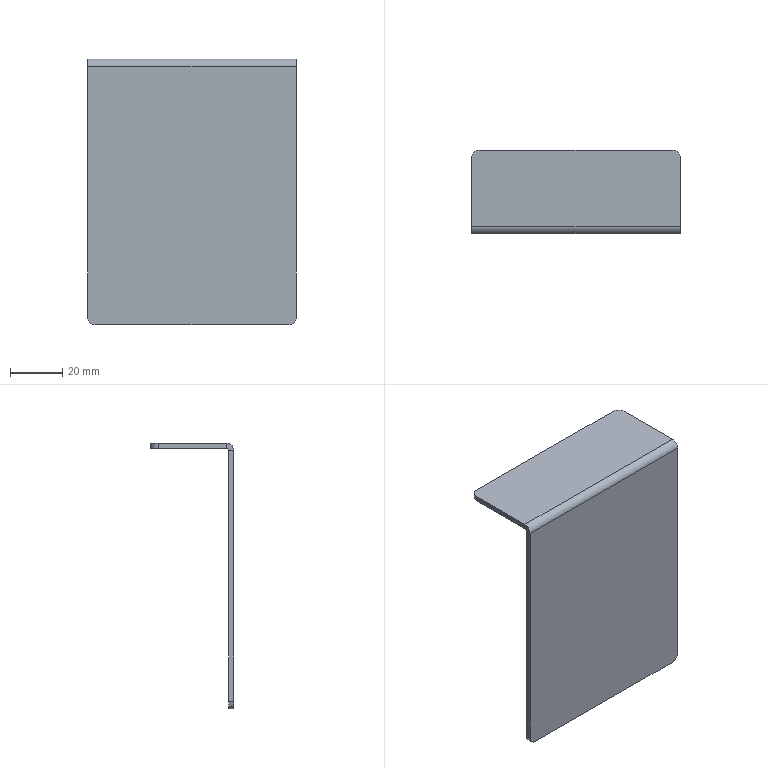Part | SolidWorks | features Fillet 1, FlatPattern 1, SMBaseFlange 1, SheetMetal 1 | 1 solid | 18 faces | box 80 x 32 x 102 mm | volume 20981 mm3 | plane 12 | cylinder 6 | commonest cylinder face diameters 6 x4 1.6 x1 5.6 x1
STEP:
#1=CARTESIAN_POINT('',(40.,0.,-0.8));
#2=VERTEX_POINT('',#1);
#3=CARTESIAN_POINT('',(40.,-2.,-0.8));
#4=VERTEX_POINT('',#3);
#5=CARTESIAN_POINT('',(40.,0.,-0.8));
#6=DIRECTION('',(0.,-1.,0.));
#7=VECTOR('',#6,1000.);
#8=LINE('',#5,#7);
#9=EDGE_CURVE('',#2,#4,#8,.T.);
#10=ORIENTED_EDGE('',*,*,#9,.F.);
#11=CARTESIAN_POINT('',(40.,0.8,0.));
#12=VERTEX_POINT('',#11);
#13=CARTESIAN_POINT('',(40.,0.8,-0.8));
#14=DIRECTION('',(1.,0.,0.));
#15=DIRECTION('',(0.,0.,1.));
#16=AXIS2_PLACEMENT_3D('',#13,#14,#15);
#17=CIRCLE('',#16,0.8);
#18=EDGE_CURVE('',#12,#2,#17,.T.);
#19=ORIENTED_EDGE('',*,*,#18,.F.);
#20=CARTESIAN_POINT('',(40.,0.8,2.));
#21=VERTEX_POINT('',#20);
#22=CARTESIAN_POINT('',(40.,0.8,2.));
#23=DIRECTION('',(0.,0.,-1.));
#24=VECTOR('',#23,1000.);
#25=LINE('',#22,#24);
#26=EDGE_CURVE('',#21,#12,#25,.T.);
#27=ORIENTED_EDGE('',*,*,#26,.F.);
#28=CARTESIAN_POINT('',(40.,0.8,-0.8));
#29=DIRECTION('',(1.,0.,0.));
#30=DIRECTION('',(0.,0.,-1.));
#31=AXIS2_PLACEMENT_3D('',#28,#29,#30);
#32=CIRCLE('',#31,2.8);
#33=EDGE_CURVE('',#21,#4,#32,.T.);
#34=ORIENTED_EDGE('',*,*,#33,.T.);
#35=EDGE_LOOP('',(#10,#19,#27,#34));
#36=FACE_OUTER_BOUND('',#35,.T.);
#37=CARTESIAN_POINT('',(40.,0.,-0.8));
#38=DIRECTION('',(1.,0.,0.));
#39=DIRECTION('',(0.,0.,-1.));
#40=AXIS2_PLACEMENT_3D('',#37,#38,#39);
#41=PLANE('',#40);
#42=ADVANCED_FACE('',(#36),#41,.T.);
#43=CARTESIAN_POINT('',(40.,-2.,-97.));
#44=VERTEX_POINT('',#43);
#45=CARTESIAN_POINT('',(40.,-2.,0.));
#46=DIRECTION('',(0.,0.,-1.));
#47=VECTOR('',#46,1000.);
#48=LINE('',#45,#47);
#49=EDGE_CURVE('',#4,#44,#48,.T.);
#50=ORIENTED_EDGE('',*,*,#49,.T.);
#51=CARTESIAN_POINT('',(40.,0.,-97.));
#52=VERTEX_POINT('',#51);
#53=CARTESIAN_POINT('',(40.,0.8,-97.));
#54=DIRECTION('',(0.,1.,0.));
#55=VECTOR('',#54,1000.);
#56=LINE('',#53,#55);
#57=EDGE_CURVE('',#44,#52,#56,.T.);
#58=ORIENTED_EDGE('',*,*,#57,.T.);
#59=CARTESIAN_POINT('',(40.,0.,0.));
#60=DIRECTION('',(0.,0.,-1.));
#61=VECTOR('',#60,1000.);
#62=LINE('',#59,#61);
#63=EDGE_CURVE('',#2,#52,#62,.T.);
#64=ORIENTED_EDGE('',*,*,#63,.F.);
#65=ORIENTED_EDGE('',*,*,#9,.T.);
#66=EDGE_LOOP('',(#50,#58,#64,#65));
#67=FACE_OUTER_BOUND('',#66,.T.);
#68=CARTESIAN_POINT('',(40.,0.8,2.));
#69=DIRECTION('',(1.,0.,0.));
#70=DIRECTION('',(0.,0.,-1.));
#71=AXIS2_PLACEMENT_3D('',#68,#69,#70);
#72=PLANE('',#71);
#73=ADVANCED_FACE('',(#67),#72,.T.);
#74=CARTESIAN_POINT('',(-40.,0.8,0.));
#75=VERTEX_POINT('',#74);
#76=CARTESIAN_POINT('',(-40.,0.8,2.));
#77=VERTEX_POINT('',#76);
#78=CARTESIAN_POINT('',(-40.,0.8,0.));
#79=DIRECTION('',(0.,0.,1.));
#80=VECTOR('',#79,1000.);
#81=LINE('',#78,#80);
#82=EDGE_CURVE('',#75,#77,#81,.T.);
#83=ORIENTED_EDGE('',*,*,#82,.F.);
#84=CARTESIAN_POINT('',(-40.,0.,-0.8));
#85=VERTEX_POINT('',#84);
#86=CARTESIAN_POINT('',(-40.,0.8,-0.8));
#87=DIRECTION('',(1.,0.,0.));
#88=DIRECTION('',(0.,0.,1.));
#89=AXIS2_PLACEMENT_3D('',#86,#87,#88);
#90=CIRCLE('',#89,0.8);
#91=EDGE_CURVE('',#75,#85,#90,.T.);
#92=ORIENTED_EDGE('',*,*,#91,.T.);
#93=CARTESIAN_POINT('',(-40.,-2.,-0.8));
#94=VERTEX_POINT('',#93);
#95=CARTESIAN_POINT('',(-40.,-2.,-0.8));
#96=DIRECTION('',(0.,1.,0.));
#97=VECTOR('',#96,1000.);
#98=LINE('',#95,#97);
#99=EDGE_CURVE('',#94,#85,#98,.T.);
#100=ORIENTED_EDGE('',*,*,#99,.F.);
#101=CARTESIAN_POINT('',(-40.,0.8,-0.8));
#102=DIRECTION('',(1.,0.,0.));
#103=DIRECTION('',(0.,0.,-1.));
#104=AXIS2_PLACEMENT_3D('',#101,#102,#103);
#105=CIRCLE('',#104,2.8);
#106=EDGE_CURVE('',#77,#94,#105,.T.);
#107=ORIENTED_EDGE('',*,*,#106,.F.);
#108=EDGE_LOOP('',(#83,#92,#100,#107));
#109=FACE_OUTER_BOUND('',#108,.T.);
#110=CARTESIAN_POINT('',(-40.,0.8,0.));
#111=DIRECTION('',(-1.,0.,0.));
#112=DIRECTION('',(0.,0.,1.));
#113=AXIS2_PLACEMENT_3D('',#110,#111,#112);
#114=PLANE('',#113);
#115=ADVANCED_FACE('',(#109),#114,.T.);
#116=CARTESIAN_POINT('',(-40.,27.,2.));
#117=VERTEX_POINT('',#116);
#118=CARTESIAN_POINT('',(-40.,30.,2.));
#119=DIRECTION('',(0.,-1.,0.));
#120=VECTOR('',#119,1000.);
#121=LINE('',#118,#120);
#122=EDGE_CURVE('',#117,#77,#121,.T.);
#123=ORIENTED_EDGE('',*,*,#122,.F.);
#124=CARTESIAN_POINT('',(-40.,27.,0.));
#125=VERTEX_POINT('',#124);
#126=CARTESIAN_POINT('',(-40.,27.,-0.8));
#127=DIRECTION('',(0.,0.,-1.));
#128=VECTOR('',#127,1000.);
#129=LINE('',#126,#128);
#130=EDGE_CURVE('',#117,#125,#129,.T.);
#131=ORIENTED_EDGE('',*,*,#130,.T.);
#132=CARTESIAN_POINT('',(-40.,30.,0.));
#133=DIRECTION('',(0.,-1.,0.));
#134=VECTOR('',#133,1000.);
#135=LINE('',#132,#134);
#136=EDGE_CURVE('',#125,#75,#135,.T.);
#137=ORIENTED_EDGE('',*,*,#136,.T.);
#138=ORIENTED_EDGE('',*,*,#82,.T.);
#139=EDGE_LOOP('',(#123,#131,#137,#138));
#140=FACE_OUTER_BOUND('',#139,.T.);
#141=CARTESIAN_POINT('',(-40.,-2.,-0.8));
#142=DIRECTION('',(-1.,0.,0.));
#143=DIRECTION('',(0.,0.,1.));
#144=AXIS2_PLACEMENT_3D('',#141,#142,#143);
#145=PLANE('',#144);
#146=ADVANCED_FACE('',(#140),#145,.T.);
#147=CARTESIAN_POINT('',(37.,-2.,-100.));
#148=VERTEX_POINT('',#147);
#149=CARTESIAN_POINT('',(-37.,-2.,-100.));
#150=VERTEX_POINT('',#149);
#151=CARTESIAN_POINT('',(40.,-2.,-100.));
#152=DIRECTION('',(-1.,0.,0.));
#153=VECTOR('',#152,1000.);
#154=LINE('',#151,#153);
#155=EDGE_CURVE('',#148,#150,#154,.T.);
#156=ORIENTED_EDGE('',*,*,#155,.F.);
#157=CARTESIAN_POINT('',(37.,-2.,-97.));
#158=DIRECTION('',(0.,-1.,0.));
#159=DIRECTION('',(0.,0.,1.));
#160=AXIS2_PLACEMENT_3D('',#157,#158,#159);
#161=CIRCLE('',#160,3.);
#162=EDGE_CURVE('',#148,#44,#161,.T.);
#163=ORIENTED_EDGE('',*,*,#162,.T.);
#164=ORIENTED_EDGE('',*,*,#49,.F.);
#165=CARTESIAN_POINT('',(40.,-2.,-0.8));
#166=DIRECTION('',(-1.,0.,0.));
#167=VECTOR('',#166,1000.);
#168=LINE('',#165,#167);
#169=EDGE_CURVE('',#4,#94,#168,.T.);
#170=ORIENTED_EDGE('',*,*,#169,.T.);
#171=CARTESIAN_POINT('',(-40.,-2.,-97.));
#172=VERTEX_POINT('',#171);
#173=CARTESIAN_POINT('',(-40.,-2.,0.));
#174=DIRECTION('',(0.,0.,-1.));
#175=VECTOR('',#174,1000.);
#176=LINE('',#173,#175);
#177=EDGE_CURVE('',#94,#172,#176,.T.);
#178=ORIENTED_EDGE('',*,*,#177,.T.);
#179=CARTESIAN_POINT('',(-37.,-2.,-97.));
#180=DIRECTION('',(0.,-1.,0.));
#181=DIRECTION('',(0.,0.,1.));
#182=AXIS2_PLACEMENT_3D('',#179,#180,#181);
#183=CIRCLE('',#182,3.);
#184=EDGE_CURVE('',#172,#150,#183,.T.);
#185=ORIENTED_EDGE('',*,*,#184,.T.);
#186=EDGE_LOOP('',(#156,#163,#164,#170,#178,#185));
#187=FACE_OUTER_BOUND('',#186,.T.);
#188=CARTESIAN_POINT('',(40.,-2.,0.));
#189=DIRECTION('',(0.,1.,0.));
#190=DIRECTION('',(0.,0.,1.));
#191=AXIS2_PLACEMENT_3D('',#188,#189,#190);
#192=PLANE('',#191);
#193=ADVANCED_FACE('',(#187),#192,.F.);
#194=CARTESIAN_POINT('',(37.,0.,-100.));
#195=VERTEX_POINT('',#194);
#196=CARTESIAN_POINT('',(-37.,0.,-100.));
#197=VERTEX_POINT('',#196);
#198=CARTESIAN_POINT('',(40.,0.,-100.));
#199=DIRECTION('',(-1.,0.,0.));
#200=VECTOR('',#199,1000.);
#201=LINE('',#198,#200);
#202=EDGE_CURVE('',#195,#197,#201,.T.);
#203=ORIENTED_EDGE('',*,*,#202,.F.);
#204=CARTESIAN_POINT('',(37.,0.,-100.));
#205=DIRECTION('',(0.,-1.,0.));
#206=VECTOR('',#205,1000.);
#207=LINE('',#204,#206);
#208=EDGE_CURVE('',#195,#148,#207,.T.);
#209=ORIENTED_EDGE('',*,*,#208,.T.);
#210=ORIENTED_EDGE('',*,*,#155,.T.);
#211=CARTESIAN_POINT('',(-37.,0.,-100.));
#212=DIRECTION('',(0.,1.,0.));
#213=VECTOR('',#212,1000.);
#214=LINE('',#211,#213);
#215=EDGE_CURVE('',#150,#197,#214,.T.);
#216=ORIENTED_EDGE('',*,*,#215,.T.);
#217=EDGE_LOOP('',(#203,#209,#210,#216));
#218=FACE_OUTER_BOUND('',#217,.T.);
#219=CARTESIAN_POINT('',(40.,0.,-100.));
#220=DIRECTION('',(0.,0.,-1.));
#221=DIRECTION('',(-1.,0.,0.));
#222=AXIS2_PLACEMENT_3D('',#219,#220,#221);
#223=PLANE('',#222);
#224=ADVANCED_FACE('',(#218),#223,.T.);
#225=ORIENTED_EDGE('',*,*,#63,.T.);
#226=CARTESIAN_POINT('',(37.,0.,-97.));
#227=DIRECTION('',(0.,1.,0.));
#228=DIRECTION('',(0.,0.,1.));
#229=AXIS2_PLACEMENT_3D('',#226,#227,#228);
#230=CIRCLE('',#229,3.);
#231=EDGE_CURVE('',#52,#195,#230,.T.);
#232=ORIENTED_EDGE('',*,*,#231,.T.);
#233=ORIENTED_EDGE('',*,*,#202,.T.);
#234=CARTESIAN_POINT('',(-40.,0.,-97.));
#235=VERTEX_POINT('',#234);
#236=CARTESIAN_POINT('',(-37.,0.,-97.));
#237=DIRECTION('',(0.,1.,0.));
#238=DIRECTION('',(0.,0.,1.));
#239=AXIS2_PLACEMENT_3D('',#236,#237,#238);
#240=CIRCLE('',#239,3.);
#241=EDGE_CURVE('',#197,#235,#240,.T.);
#242=ORIENTED_EDGE('',*,*,#241,.T.);
#243=CARTESIAN_POINT('',(-40.,0.,0.));
#244=DIRECTION('',(0.,0.,-1.));
#245=VECTOR('',#244,1000.);
#246=LINE('',#243,#245);
#247=EDGE_CURVE('',#85,#235,#246,.T.);
#248=ORIENTED_EDGE('',*,*,#247,.F.);
#249=CARTESIAN_POINT('',(40.,0.,-0.8));
#250=DIRECTION('',(-1.,0.,0.));
#251=VECTOR('',#250,1000.);
#252=LINE('',#249,#251);
#253=EDGE_CURVE('',#2,#85,#252,.T.);
#254=ORIENTED_EDGE('',*,*,#253,.F.);
#255=EDGE_LOOP('',(#225,#232,#233,#242,#248,#254));
#256=FACE_OUTER_BOUND('',#255,.T.);
#257=CARTESIAN_POINT('',(40.,0.,0.));
#258=DIRECTION('',(0.,1.,0.));
#259=DIRECTION('',(0.,0.,1.));
#260=AXIS2_PLACEMENT_3D('',#257,#258,#259);
#261=PLANE('',#260);
#262=ADVANCED_FACE('',(#256),#261,.T.);
#263=ORIENTED_EDGE('',*,*,#91,.F.);
#264=CARTESIAN_POINT('',(40.,0.8,0.));
#265=DIRECTION('',(-1.,0.,0.));
#266=VECTOR('',#265,1000.);
#267=LINE('',#264,#266);
#268=EDGE_CURVE('',#12,#75,#267,.T.);
#269=ORIENTED_EDGE('',*,*,#268,.F.);
#270=ORIENTED_EDGE('',*,*,#18,.T.);
#271=ORIENTED_EDGE('',*,*,#253,.T.);
#272=EDGE_LOOP('',(#263,#269,#270,#271));
#273=FACE_OUTER_BOUND('',#272,.T.);
#274=CARTESIAN_POINT('',(40.,0.8,-0.8));
#275=DIRECTION('',(-1.,0.,0.));
#276=DIRECTION('',(0.,0.,1.));
#277=AXIS2_PLACEMENT_3D('',#274,#275,#276);
#278=CYLINDRICAL_SURFACE('',#277,0.8);
#279=ADVANCED_FACE('',(#273),#278,.F.);
#280=ORIENTED_EDGE('',*,*,#136,.F.);
#281=CARTESIAN_POINT('',(-37.,30.,0.));
#282=VERTEX_POINT('',#281);
#283=CARTESIAN_POINT('',(-37.,27.,0.));
#284=DIRECTION('',(0.,0.,-1.));
#285=DIRECTION('',(0.,1.,0.));
#286=AXIS2_PLACEMENT_3D('',#283,#284,#285);
#287=CIRCLE('',#286,3.);
#288=EDGE_CURVE('',#125,#282,#287,.T.);
#289=ORIENTED_EDGE('',*,*,#288,.T.);
#290=CARTESIAN_POINT('',(37.,30.,0.));
#291=VERTEX_POINT('',#290);
#292=CARTESIAN_POINT('',(40.,30.,0.));
#293=DIRECTION('',(-1.,0.,0.));
#294=VECTOR('',#293,1000.);
#295=LINE('',#292,#294);
#296=EDGE_CURVE('',#291,#282,#295,.T.);
#297=ORIENTED_EDGE('',*,*,#296,.F.);
#298=CARTESIAN_POINT('',(40.,27.,0.));
#299=VERTEX_POINT('',#298);
#300=CARTESIAN_POINT('',(37.,27.,0.));
#301=DIRECTION('',(0.,0.,-1.));
#302=DIRECTION('',(0.,1.,0.));
#303=AXIS2_PLACEMENT_3D('',#300,#301,#302);
#304=CIRCLE('',#303,3.);
#305=EDGE_CURVE('',#291,#299,#304,.T.);
#306=ORIENTED_EDGE('',*,*,#305,.T.);
#307=CARTESIAN_POINT('',(40.,30.,0.));
#308=DIRECTION('',(0.,-1.,0.));
#309=VECTOR('',#308,1000.);
#310=LINE('',#307,#309);
#311=EDGE_CURVE('',#299,#12,#310,.T.);
#312=ORIENTED_EDGE('',*,*,#311,.T.);
#313=ORIENTED_EDGE('',*,*,#268,.T.);
#314=EDGE_LOOP('',(#280,#289,#297,#306,#312,#313));
#315=FACE_OUTER_BOUND('',#314,.T.);
#316=CARTESIAN_POINT('',(40.,30.,0.));
#317=DIRECTION('',(0.,0.,-1.));
#318=DIRECTION('',(0.,1.,0.));
#319=AXIS2_PLACEMENT_3D('',#316,#317,#318);
#320=PLANE('',#319);
#321=ADVANCED_FACE('',(#315),#320,.T.);
#322=ORIENTED_EDGE('',*,*,#296,.T.);
#323=CARTESIAN_POINT('',(-37.,30.,2.));
#324=VERTEX_POINT('',#323);
#325=CARTESIAN_POINT('',(-37.,30.,2.));
#326=DIRECTION('',(0.,0.,1.));
#327=VECTOR('',#326,1000.);
#328=LINE('',#325,#327);
#329=EDGE_CURVE('',#282,#324,#328,.T.);
#330=ORIENTED_EDGE('',*,*,#329,.T.);
#331=CARTESIAN_POINT('',(37.,30.,2.));
#332=VERTEX_POINT('',#331);
#333=CARTESIAN_POINT('',(40.,30.,2.));
#334=DIRECTION('',(-1.,0.,0.));
#335=VECTOR('',#334,1000.);
#336=LINE('',#333,#335);
#337=EDGE_CURVE('',#332,#324,#336,.T.);
#338=ORIENTED_EDGE('',*,*,#337,.F.);
#339=CARTESIAN_POINT('',(37.,30.,0.));
#340=DIRECTION('',(0.,0.,-1.));
#341=VECTOR('',#340,1000.);
#342=LINE('',#339,#341);
#343=EDGE_CURVE('',#332,#291,#342,.T.);
#344=ORIENTED_EDGE('',*,*,#343,.T.);
#345=EDGE_LOOP('',(#322,#330,#338,#344));
#346=FACE_OUTER_BOUND('',#345,.T.);
#347=CARTESIAN_POINT('',(40.,30.,2.));
#348=DIRECTION('',(0.,1.,0.));
#349=DIRECTION('',(0.,0.,1.));
#350=AXIS2_PLACEMENT_3D('',#347,#348,#349);
#351=PLANE('',#350);
#352=ADVANCED_FACE('',(#346),#351,.T.);
#353=ORIENTED_EDGE('',*,*,#337,.T.);
#354=CARTESIAN_POINT('',(-37.,27.,2.));
#355=DIRECTION('',(0.,0.,1.));
#356=DIRECTION('',(0.,1.,0.));
#357=AXIS2_PLACEMENT_3D('',#354,#355,#356);
#358=CIRCLE('',#357,3.);
#359=EDGE_CURVE('',#324,#117,#358,.T.);
#360=ORIENTED_EDGE('',*,*,#359,.T.);
#361=ORIENTED_EDGE('',*,*,#122,.T.);
#362=CARTESIAN_POINT('',(40.,0.8,2.));
#363=DIRECTION('',(-1.,0.,0.));
#364=VECTOR('',#363,1000.);
#365=LINE('',#362,#364);
#366=EDGE_CURVE('',#21,#77,#365,.T.);
#367=ORIENTED_EDGE('',*,*,#366,.F.);
#368=CARTESIAN_POINT('',(40.,27.,2.));
#369=VERTEX_POINT('',#368);
#370=CARTESIAN_POINT('',(40.,30.,2.));
#371=DIRECTION('',(0.,-1.,0.));
#372=VECTOR('',#371,1000.);
#373=LINE('',#370,#372);
#374=EDGE_CURVE('',#369,#21,#373,.T.);
#375=ORIENTED_EDGE('',*,*,#374,.F.);
#376=CARTESIAN_POINT('',(37.,27.,2.));
#377=DIRECTION('',(0.,0.,1.));
#378=DIRECTION('',(0.,1.,0.));
#379=AXIS2_PLACEMENT_3D('',#376,#377,#378);
#380=CIRCLE('',#379,3.);
#381=EDGE_CURVE('',#369,#332,#380,.T.);
#382=ORIENTED_EDGE('',*,*,#381,.T.);
#383=EDGE_LOOP('',(#353,#360,#361,#367,#375,#382));
#384=FACE_OUTER_BOUND('',#383,.T.);
#385=CARTESIAN_POINT('',(40.,30.,2.));
#386=DIRECTION('',(0.,0.,-1.));
#387=DIRECTION('',(0.,1.,0.));
#388=AXIS2_PLACEMENT_3D('',#385,#386,#387);
#389=PLANE('',#388);
#390=ADVANCED_FACE('',(#384),#389,.F.);
#391=ORIENTED_EDGE('',*,*,#106,.T.);
#392=ORIENTED_EDGE('',*,*,#169,.F.);
#393=ORIENTED_EDGE('',*,*,#33,.F.);
#394=ORIENTED_EDGE('',*,*,#366,.T.);
#395=EDGE_LOOP('',(#391,#392,#393,#394));
#396=FACE_OUTER_BOUND('',#395,.T.);
#397=CARTESIAN_POINT('',(40.,0.8,-0.8));
#398=DIRECTION('',(-1.,0.,0.));
#399=DIRECTION('',(0.,0.,1.));
#400=AXIS2_PLACEMENT_3D('',#397,#398,#399);
#401=CYLINDRICAL_SURFACE('',#400,2.8);
#402=ADVANCED_FACE('',(#396),#401,.T.);
#403=ORIENTED_EDGE('',*,*,#311,.F.);
#404=CARTESIAN_POINT('',(40.,27.,2.));
#405=DIRECTION('',(0.,0.,1.));
#406=VECTOR('',#405,1000.);
#407=LINE('',#404,#406);
#408=EDGE_CURVE('',#299,#369,#407,.T.);
#409=ORIENTED_EDGE('',*,*,#408,.T.);
#410=ORIENTED_EDGE('',*,*,#374,.T.);
#411=ORIENTED_EDGE('',*,*,#26,.T.);
#412=EDGE_LOOP('',(#403,#409,#410,#411));
#413=FACE_OUTER_BOUND('',#412,.T.);
#414=CARTESIAN_POINT('',(40.,0.8,-0.8));
#415=DIRECTION('',(-1.,0.,0.));
#416=DIRECTION('',(0.,0.,1.));
#417=AXIS2_PLACEMENT_3D('',#414,#415,#416);
#418=PLANE('',#417);
#419=ADVANCED_FACE('',(#413),#418,.F.);
#420=ORIENTED_EDGE('',*,*,#247,.T.);
#421=CARTESIAN_POINT('',(-40.,0.8,-97.));
#422=DIRECTION('',(0.,-1.,0.));
#423=VECTOR('',#422,1000.);
#424=LINE('',#421,#423);
#425=EDGE_CURVE('',#235,#172,#424,.T.);
#426=ORIENTED_EDGE('',*,*,#425,.T.);
#427=ORIENTED_EDGE('',*,*,#177,.F.);
#428=ORIENTED_EDGE('',*,*,#99,.T.);
#429=EDGE_LOOP('',(#420,#426,#427,#428));
#430=FACE_OUTER_BOUND('',#429,.T.);
#431=CARTESIAN_POINT('',(-40.,0.8,-0.8));
#432=DIRECTION('',(-1.,0.,0.));
#433=DIRECTION('',(0.,0.,1.));
#434=AXIS2_PLACEMENT_3D('',#431,#432,#433);
#435=PLANE('',#434);
#436=ADVANCED_FACE('',(#430),#435,.T.);
#437=ORIENTED_EDGE('',*,*,#231,.F.);
#438=ORIENTED_EDGE('',*,*,#57,.F.);
#439=ORIENTED_EDGE('',*,*,#162,.F.);
#440=ORIENTED_EDGE('',*,*,#208,.F.);
#441=EDGE_LOOP('',(#437,#438,#439,#440));
#442=FACE_OUTER_BOUND('',#441,.T.);
#443=CARTESIAN_POINT('',(37.,0.,-97.));
#444=DIRECTION('',(0.,-1.,0.));
#445=DIRECTION('',(0.,0.,-1.));
#446=AXIS2_PLACEMENT_3D('',#443,#444,#445);
#447=CYLINDRICAL_SURFACE('',#446,3.);
#448=ADVANCED_FACE('',(#442),#447,.T.);
#449=ORIENTED_EDGE('',*,*,#241,.F.);
#450=ORIENTED_EDGE('',*,*,#215,.F.);
#451=ORIENTED_EDGE('',*,*,#184,.F.);
#452=ORIENTED_EDGE('',*,*,#425,.F.);
#453=EDGE_LOOP('',(#449,#450,#451,#452));
#454=FACE_OUTER_BOUND('',#453,.T.);
#455=CARTESIAN_POINT('',(-37.,0.8,-97.));
#456=DIRECTION('',(0.,-1.,0.));
#457=DIRECTION('',(0.,0.,-1.));
#458=AXIS2_PLACEMENT_3D('',#455,#456,#457);
#459=CYLINDRICAL_SURFACE('',#458,3.);
#460=ADVANCED_FACE('',(#454),#459,.T.);
#461=ORIENTED_EDGE('',*,*,#359,.F.);
#462=ORIENTED_EDGE('',*,*,#329,.F.);
#463=ORIENTED_EDGE('',*,*,#288,.F.);
#464=ORIENTED_EDGE('',*,*,#130,.F.);
#465=EDGE_LOOP('',(#461,#462,#463,#464));
#466=FACE_OUTER_BOUND('',#465,.T.);
#467=CARTESIAN_POINT('',(-37.,27.,-0.8));
#468=DIRECTION('',(0.,0.,-1.));
#469=DIRECTION('',(-1.,0.,0.));
#470=AXIS2_PLACEMENT_3D('',#467,#468,#469);
#471=CYLINDRICAL_SURFACE('',#470,3.);
#472=ADVANCED_FACE('',(#466),#471,.T.);
#473=ORIENTED_EDGE('',*,*,#381,.F.);
#474=ORIENTED_EDGE('',*,*,#408,.F.);
#475=ORIENTED_EDGE('',*,*,#305,.F.);
#476=ORIENTED_EDGE('',*,*,#343,.F.);
#477=EDGE_LOOP('',(#473,#474,#475,#476));
#478=FACE_OUTER_BOUND('',#477,.T.);
#479=CARTESIAN_POINT('',(37.,27.,2.));
#480=DIRECTION('',(0.,0.,1.));
#481=DIRECTION('',(1.,0.,0.));
#482=AXIS2_PLACEMENT_3D('',#479,#480,#481);
#483=CYLINDRICAL_SURFACE('',#482,3.);
#484=ADVANCED_FACE('',(#478),#483,.T.);
#485=CLOSED_SHELL('',(#42,#73,#115,#146,#193,#224,#262,#279,#321,#352,#390,#402,#419,#436,#448,#460,#472,#484));
#486=MANIFOLD_SOLID_BREP('',#485);
#487=CARTESIAN_POINT('',(0.,0.,0.));
#488=DIRECTION('',(0.,0.,1.));
#489=DIRECTION('',(1.,0.,0.));
#490=AXIS2_PLACEMENT_3D('',#487,#488,#489);
#491=(LENGTH_UNIT()NAMED_UNIT(*)SI_UNIT(.MILLI.,.METRE.));
#492=UNCERTAINTY_MEASURE_WITH_UNIT(LENGTH_MEASURE(0.00001),#491,'','');
#493=(NAMED_UNIT(*)PLANE_ANGLE_UNIT()SI_UNIT($,.RADIAN.));
#494=(NAMED_UNIT(*)SI_UNIT($,.STERADIAN.)SOLID_ANGLE_UNIT());
#495=(GEOMETRIC_REPRESENTATION_CONTEXT(3)GLOBAL_UNCERTAINTY_ASSIGNED_CONTEXT((#492))GLOBAL_UNIT_ASSIGNED_CONTEXT((#491,#493,#494))REPRESENTATION_CONTEXT('',''));
#496=ADVANCED_BREP_SHAPE_REPRESENTATION('',(#486,#490),#495);